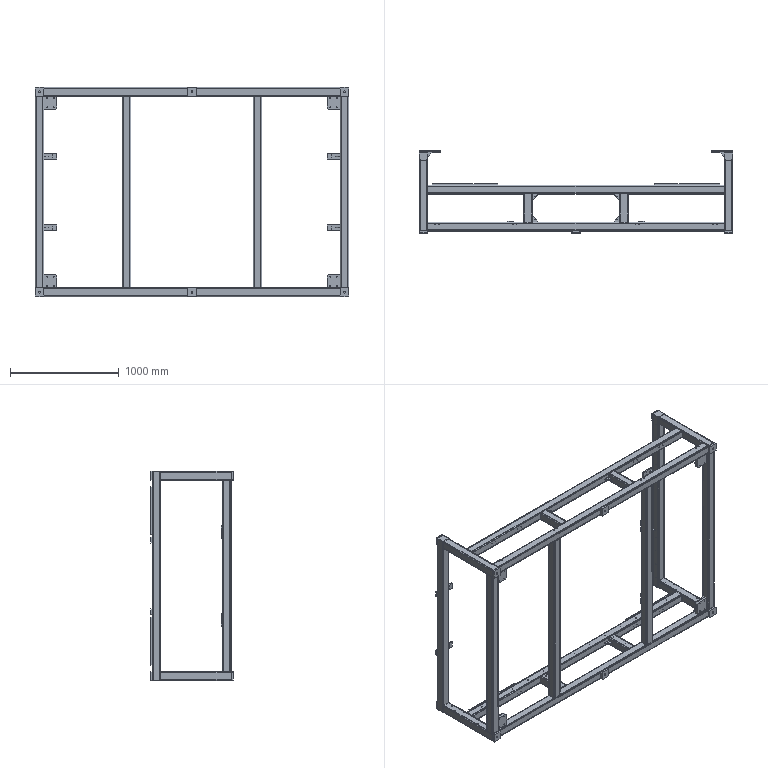Part | SolidWorks | features BaseBody 72 | 72 solids | 1552 faces | box 2880 x 757 x 1920 mm | volume 41526800 mm3 | cylinder 908 | plane 644 | commonest cylinder face diameters 6.8 x384 5 x140 3.3 x116 20 x88 10 x72 2.5 x64